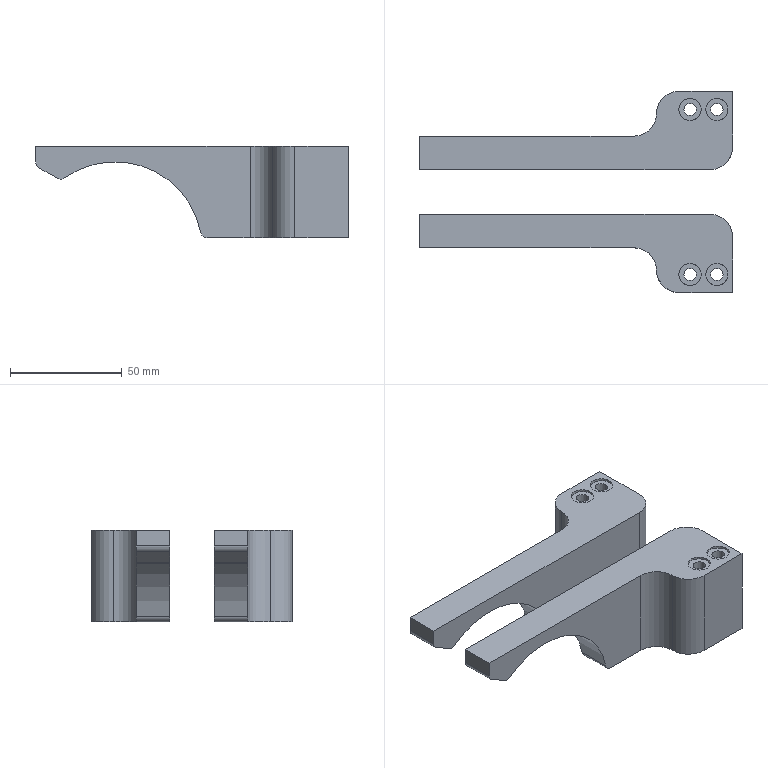NC program | NX | posted with a generic post | part box 140 x 90 x 41 mm
Lines 5892 to 6729 of 29499:
(FIXED_CONTOUR_COPY , TOOL : R4)
N11740 T08 M6
N11742 G54
N11744 G17 G0 G90 X6.198 Y17.997 S9500 M3
N11746 G43 Z30. H8
N11748 Z4.4
N11750 G94 G1 Z0.371 F3000.
N11752 X6.29 Y17.904 Z0.209
N11754 X6.41 Y17.785 Z0.086
N11756 X6.548 Y17.647 Z0.011
N11758 X6.695 Y17.5 Z-0.011
N11760 X6.831 Y17.363 Z-0.006
N11762 Y17.227 Z-0.004
N11764 X6.558 Y17.5 Z-0.014
N11766 X6.421 Z-0.017
N11768 X6.831 Y17.09 Z-0.004
N11770 Y16.954
N11772 X6.589 Y17.196 Z-0.009
N11774 X6.427 Y17.358 Z-0.015
N11776 X6.285 Y17.5 Z-0.028
N11778 X6.148 Z-0.039
N11780 X6.427 Y17.221 Z-0.013
N11782 X6.831 Y16.817 Z-0.004
N11784 Y16.682
N11786 X6.427 Y17.086 Z-0.013
N11788 X6.145 Y17.368 Z-0.037
N11790 X6.013 Y17.5 Z-0.055
N11792 X5.877 Z-0.071
N11794 X6.181 Y17.196 Z-0.032
N11796 X6.427 Y16.95 Z-0.013
N11798 X6.831 Y16.546 Z-0.004
N11800 Y16.409
N11802 X6.427 Y16.813 Z-0.013
N11804 X6.145 Y17.095 Z-0.035
N11806 X5.863 Y17.377 Z-0.07
N11808 X5.74 Y17.5 Z-0.092
N11810 X5.605 Z-0.115
N11812 X5.863 Y17.241 Z-0.068
N11814 X6.145 Y16.959 Z-0.035
N11816 X6.427 Y16.678 Z-0.013
N11818 X6.831 Y16.274 Z-0.004
N11820 Y16.14
N11822 X6.427 Y16.544 Z-0.013
N11824 X6.145 Y16.826 Z-0.035
N11826 X5.863 Y17.108 Z-0.068
N11828 X5.582 Y17.389 Z-0.117
N11830 X5.471 Y17.5 Z-0.144
N11832 X5.336 Z-0.174
N11834 X5.582 Y17.254 Z-0.115
N11836 X5.863 Y16.973 Z-0.068
N11838 X6.145 Y16.691 Z-0.035
N11840 X6.427 Y16.409 Z-0.013
N11842 X6.831 Y16.005 Z-0.004
N11844 Y15.87
N11846 X6.427 Y16.274 Z-0.013
N11848 X6.145 Y16.555 Z-0.035
N11850 X5.863 Y16.837 Z-0.068
N11852 X5.582 Y17.119 Z-0.114
N11854 X5.201 Y17.5 Z-0.206
N11856 X5.065 Z-0.238
N11858 X5.369 Y17.196 Z-0.163
N11860 X5.582 Y16.983 Z-0.114
N11862 X5.863 Y16.702 Z-0.068
N11864 X6.145 Y16.42 Z-0.035
N11866 X6.427 Y16.138 Z-0.013
N11868 X6.831 Y15.734 Z-0.004
N11870 Y15.599
N11872 X6.427 Y16.003 Z-0.013
N11874 X6.145 Y16.285 Z-0.035
N11876 X5.863 Y16.567 Z-0.068
N11878 X5.582 Y16.848 Z-0.114
N11880 X5.234 Y17.196 Z-0.194
N11882 X5.018 Y17.412 Z-0.247
N11884 X4.93 Y17.5 Z-0.273
N11886 X4.795 Z-0.309
N11888 X5.018 Y17.277 Z-0.245
N11890 X5.3 Y16.996 Z-0.178
N11892 X5.582 Y16.714 Z-0.114
N11894 X5.863 Y16.432 Z-0.068
N11896 X6.145 Y16.15 Z-0.035
N11898 X6.427 Y15.869 Z-0.013
N11900 X6.831 Y15.464 Z-0.004
N11902 Y15.333
N11904 X6.427 Y15.737 Z-0.013
N11906 X6.145 Y16.018 Z-0.035
N11908 X5.863 Y16.3 Z-0.068
N11910 X5.582 Y16.582 Z-0.114
N11912 X5.018 Y17.145 Z-0.244
N11914 X4.736 Y17.427 Z-0.324
N11916 X4.664 Y17.5 Z-0.351
N11918 X4.531 Z-0.398
N11920 X4.736 Y17.295 Z-0.322
N11922 X5.018 Y17.013 Z-0.244
N11924 X5.582 Y16.449 Z-0.114
N11926 X5.863 Y16.168 Z-0.068
N11928 X6.145 Y15.886 Z-0.035
N11930 X6.427 Y15.604 Z-0.013
N11932 X6.831 Y15.2 Z-0.004
N11934 Y15.067
N11936 X6.427 Y15.471 Z-0.013
N11938 X6.145 Y15.753 Z-0.035
N11940 X5.863 Y16.034 Z-0.068
N11942 X5.582 Y16.316 Z-0.114
N11944 X5.018 Y16.88 Z-0.244
N11946 X4.736 Y17.161 Z-0.321
N11948 X4.455 Y17.443 Z-0.424
N11950 X4.398 Y17.5 Z-0.448
N11952 X4.265 Z-0.501
N11954 X4.455 Y17.311 Z-0.422
N11956 X4.736 Y17.029 Z-0.321
N11958 X5.018 Y16.747 Z-0.244
N11960 X5.582 Y16.184 Z-0.114
N11962 X5.863 Y15.902 Z-0.068
N11964 X6.145 Y15.62 Z-0.035
N11966 X6.427 Y15.338 Z-0.013
N11968 X6.831 Y14.934 Z-0.004
N11970 Y14.802
N11972 X6.427 Y15.206 Z-0.013
N11974 X6.145 Y15.488 Z-0.035
N11976 X5.863 Y15.77 Z-0.068
N11978 X5.582 Y16.051 Z-0.114
N11980 X5.018 Y16.615 Z-0.244
N11982 X4.736 Y16.897 Z-0.321
N11984 X4.437 Y17.196 Z-0.427
N11986 X4.133 Y17.5 Z-0.555
N11988 X4.002 Z-0.608
N11990 X4.306 Y17.196 Z-0.48
N11992 X4.455 Y17.047 Z-0.42
N11994 X4.736 Y16.766 Z-0.321
N11996 X5.018 Y16.484 Z-0.244
N11998 X5.582 Y15.92 Z-0.114
N12000 X5.863 Y15.639 Z-0.068
N12002 X6.145 Y15.357 Z-0.035
N12004 X6.427 Y15.075 Z-0.013
N12006 X6.831 Y14.671 Z-0.004
N12008 Y14.541
N12010 X6.427 Y14.945 Z-0.013
N12012 X6.145 Y15.227 Z-0.035
N12014 X5.863 Y15.509 Z-0.068
N12016 X5.582 Y15.791 Z-0.114
N12018 X5.018 Y16.354 Z-0.244
N12020 X4.736 Y16.636 Z-0.321
N12022 X4.455 Y16.918 Z-0.42
N12024 X4.176 Y17.196 Z-0.532
N12026 X3.891 Y17.481 Z-0.654
N12028 X3.872 Y17.5 Z-0.663
N12030 X3.744 Z-0.726
N12032 X3.891 Y17.353 Z-0.652
N12034 X4.173 Y17.071 Z-0.534
N12036 X4.455 Y16.79 Z-0.42
N12038 X4.736 Y16.508 Z-0.321
N12040 X5.018 Y16.226 Z-0.244
N12042 X5.582 Y15.663 Z-0.114
N12044 X5.863 Y15.381 Z-0.068
N12046 X6.145 Y15.099 Z-0.035
N12048 X6.427 Y14.817 Z-0.013
N12050 X6.831 Y14.413 Z-0.004
N12052 Y14.283
N12054 X6.427 Y14.687 Z-0.013
N12056 X6.145 Y14.969 Z-0.035
N12058 X5.863 Y15.251 Z-0.068
N12060 X5.582 Y15.532 Z-0.114
N12062 X5.02 Y16.094 Z-0.244
N12064 X4.736 Y16.378 Z-0.321
N12066 X4.455 Y16.659 Z-0.42
N12068 X3.891 Y17.223 Z-0.65
N12070 X3.614 Y17.5 Z-0.785
N12072 X3.487 Z-0.858
N12074 X3.609 Y17.377 Z-0.787
N12076 X3.891 Y17.096 Z-0.649
N12078 X4.455 Y16.532 Z-0.42
N12080 X4.736 Y16.25 Z-0.321
N12082 X5.018 Y15.969 Z-0.244
N12084 X5.582 Y15.405 Z-0.114
N12086 X5.863 Y15.123 Z-0.068
N12088 X6.145 Y14.842 Z-0.035
N12090 X6.427 Y14.56 Z-0.013
N12092 X6.831 Y14.156 Z-0.004
N12094 Y14.032
N12096 X6.427 Y14.437 Z-0.013
N12098 X6.145 Y14.718 Z-0.035
N12100 X5.863 Y15. Z-0.068
N12102 X5.582 Y15.282 Z-0.114
N12104 X5.018 Y15.845 Z-0.244
N12106 X4.736 Y16.127 Z-0.321
N12108 X4.455 Y16.409 Z-0.42
N12110 X3.891 Y16.972 Z-0.649
N12112 X3.609 Y17.254 Z-0.787
N12114 X3.363 Y17.5 Z-0.93
N12116 X3.237 Z-1.004
N12118 X3.327 Y17.41 Z-0.95
N12120 X3.609 Y17.128 Z-0.787
N12122 X3.891 Y16.846 Z-0.649
N12124 X4.455 Y16.283 Z-0.42
N12126 X4.736 Y16.001 Z-0.321
N12128 X5.018 Y15.719 Z-0.244
N12130 X5.582 Y15.156 Z-0.114
N12132 X5.863 Y14.874 Z-0.068
N12134 X6.145 Y14.592 Z-0.035
N12136 X6.427 Y14.31 Z-0.013
N12138 X6.831 Y13.906 Z-0.004
N12140 Y13.779
N12142 X6.427 Y14.183 Z-0.013
N12144 X6.145 Y14.465 Z-0.035
N12146 X5.863 Y14.747 Z-0.068
N12148 X5.582 Y15.029 Z-0.114
N12150 X5.018 Y15.592 Z-0.244
N12152 X4.736 Y15.874 Z-0.321
N12154 X4.455 Y16.156 Z-0.42
N12156 X3.891 Y16.719 Z-0.649
N12158 X3.609 Y17.001 Z-0.787
N12160 X3.327 Y17.283 Z-0.95
N12162 X3.11 Y17.5 Z-1.08
N12164 X3.046 Z-1.118
N12166 X2.985 Z-1.16
N12168 X3.046 Y17.439 Z-1.117
N12170 X3.327 Y17.157 Z-0.95
N12172 X3.609 Y16.875 Z-0.787
N12174 X3.891 Y16.593 Z-0.649
N12176 X4.455 Y16.03 Z-0.42
N12178 X4.736 Y15.748 Z-0.321
N12180 X5.018 Y15.466 Z-0.244
N12182 X5.582 Y14.903 Z-0.114
N12184 X5.863 Y14.621 Z-0.068
N12186 X6.145 Y14.339 Z-0.035
N12188 X6.427 Y14.058 Z-0.013
N12190 X6.831 Y13.653 Z-0.004
N12192 Y13.531
N12194 X6.427 Y13.935 Z-0.013
N12196 X6.145 Y14.217 Z-0.035
N12198 X5.863 Y14.499 Z-0.068
N12200 X5.582 Y14.781 Z-0.114
N12202 X5.018 Y15.344 Z-0.244
N12204 X4.736 Y15.626 Z-0.321
N12206 X4.455 Y15.908 Z-0.42
N12208 X3.891 Y16.471 Z-0.649
N12210 X3.609 Y16.753 Z-0.787
N12212 X3.327 Y17.035 Z-0.95
N12214 X3.046 Y17.317 Z-1.117
N12216 X2.967 Y17.395 Z-1.169
N12218 X2.862 Y17.5 Z-1.243
N12220 X2.764 Z-1.308
N12222 X2.74 Z-1.327
N12224 X2.764 Y17.476 Z-1.308
N12226 X2.858 Y17.381 Z-1.244
N12228 X2.905 Y17.335 Z-1.21
N12230 X3.046 Y17.194 Z-1.117
N12232 X3.327 Y16.912 Z-0.95
N12234 X3.609 Y16.631 Z-0.787
N12236 X3.891 Y16.349 Z-0.649
N12238 X4.455 Y15.785 Z-0.42
N12240 X4.736 Y15.504 Z-0.321
N12242 X5.018 Y15.222 Z-0.244
N12244 X5.582 Y14.658 Z-0.114
N12246 X5.863 Y14.376 Z-0.068
N12248 X6.145 Y14.095 Z-0.035
N12250 X6.427 Y13.813 Z-0.013
N12252 X6.831 Y13.409 Z-0.004
N12254 Y13.289
N12256 X6.427 Y13.693 Z-0.013
N12258 X6.145 Y13.975 Z-0.035
N12260 X5.863 Y14.257 Z-0.068
N12262 X5.582 Y14.539 Z-0.114
N12264 X5.018 Y15.102 Z-0.244
N12266 X4.736 Y15.384 Z-0.321
N12268 X4.455 Y15.666 Z-0.42
N12270 X3.891 Y16.229 Z-0.649
N12272 X3.609 Y16.511 Z-0.787
N12274 X3.327 Y16.793 Z-0.95
N12276 X3.046 Y17.075 Z-1.117
N12278 X2.845 Y17.275 Z-1.25
N12280 X2.764 Y17.356 Z-1.306
N12282 X2.62 Y17.5 Z-1.422
N12284 X2.502 Z-1.512
N12286 X2.764 Y17.238 Z-1.304
N12288 X3.046 Y16.956 Z-1.117
N12290 X3.327 Y16.675 Z-0.95
N12292 X3.609 Y16.393 Z-0.787
N12294 X3.891 Y16.111 Z-0.649
N12296 X4.455 Y15.548 Z-0.42
N12298 X4.736 Y15.266 Z-0.321
N12300 X5.02 Y14.982 Z-0.244
N12302 X5.582 Y14.42 Z-0.114
N12304 X5.863 Y14.139 Z-0.068
N12306 X6.145 Y13.857 Z-0.035
N12308 X6.427 Y13.575 Z-0.013
N12310 X6.831 Y13.171 Z-0.004
N12312 Y13.057
N12314 X6.427 Y13.461 Z-0.013
N12316 X6.145 Y13.743 Z-0.035
N12318 X5.863 Y14.025 Z-0.068
N12320 X5.582 Y14.307 Z-0.114
N12322 X5.018 Y14.87 Z-0.244
N12324 X4.736 Y15.152 Z-0.321
N12326 X4.455 Y15.434 Z-0.42
N12328 X3.891 Y15.997 Z-0.649
N12330 X3.609 Y16.279 Z-0.787
N12332 X3.327 Y16.561 Z-0.95
N12334 X3.046 Y16.843 Z-1.117
N12336 X2.764 Y17.124 Z-1.303
N12338 X2.451 Y17.438 Z-1.551
N12340 X2.388 Y17.5 Z-1.604
N12342 X2.27 Z-1.701
N12344 X2.482 Y17.288 Z-1.525
N12346 X2.764 Y17.006 Z-1.303
N12348 X3.046 Y16.724 Z-1.117
N12350 X3.327 Y16.442 Z-0.95
N12352 X3.609 Y16.161 Z-0.787
N12354 X3.891 Y15.879 Z-0.649
N12356 X4.455 Y15.315 Z-0.42
N12358 X4.736 Y15.033 Z-0.321
N12360 X5.018 Y14.752 Z-0.244
N12362 X5.582 Y14.188 Z-0.114
N12364 X5.863 Y13.906 Z-0.068
N12366 X6.145 Y13.625 Z-0.035
N12368 X6.427 Y13.343 Z-0.013
N12370 X6.831 Y12.939 Z-0.004
N12372 Y12.82
N12374 X6.427 Y13.224 Z-0.013
N12376 X6.145 Y13.505 Z-0.035
N12378 X5.863 Y13.787 Z-0.068
N12380 X5.582 Y14.069 Z-0.114
N12382 X5.018 Y14.633 Z-0.244
N12384 X4.736 Y14.914 Z-0.321
N12386 X4.455 Y15.196 Z-0.42
N12388 X3.891 Y15.76 Z-0.649
N12390 X3.609 Y16.041 Z-0.787
N12392 X3.327 Y16.323 Z-0.95
N12394 X3.046 Y16.605 Z-1.117
N12396 X2.764 Y16.887 Z-1.303
N12398 X2.482 Y17.168 Z-1.525
N12400 X2.189 Y17.461 Z-1.766
N12402 X2.151 Y17.5 Z-1.803
N12404 X2.032 Z-1.907
N12406 X2.06 Y17.472 Z-1.879
N12408 X2.2 Y17.331 Z-1.757
N12410 X2.482 Y17.049 Z-1.525
N12412 X2.764 Y16.768 Z-1.303
N12414 X3.046 Y16.486 Z-1.117
N12416 X3.327 Y16.204 Z-0.95
N12418 X3.609 Y15.922 Z-0.787
N12420 X3.891 Y15.641 Z-0.649
N12422 X4.455 Y15.077 Z-0.42
N12424 X4.736 Y14.795 Z-0.321
N12426 X5.018 Y14.514 Z-0.244
N12428 X5.582 Y13.95 Z-0.114
N12430 X5.863 Y13.668 Z-0.068
N12432 X6.145 Y13.386 Z-0.035
N12434 X6.427 Y13.105 Z-0.013
N12436 X6.831 Y12.701 Z-0.004
N12438 Y12.587
N12440 X6.427 Y12.991 Z-0.013
N12442 X6.145 Y13.272 Z-0.035
N12444 X5.863 Y13.554 Z-0.068
N12446 X5.582 Y13.836 Z-0.114
N12448 X5.018 Y14.4 Z-0.244
N12450 X4.736 Y14.681 Z-0.321
N12452 X4.455 Y14.963 Z-0.42
N12454 X3.891 Y15.527 Z-0.649
N12456 X3.609 Y15.808 Z-0.787
N12458 X3.329 Y16.089 Z-0.949
N12460 X3.046 Y16.372 Z-1.117
N12462 X2.764 Y16.654 Z-1.303
N12464 X2.482 Y16.935 Z-1.525
N12466 X2.178 Y17.239 Z-1.776
N12468 X1.979 Y17.439 Z-1.955
N12470 X1.917 Y17.5 Z-2.016
N12472 X1.811 Z-2.132
N12474 X1.919 Y17.392 Z-2.014
N12476 X1.985 Y17.326 Z-1.951
N12478 X2.2 Y17.11 Z-1.757
N12480 X2.482 Y16.828 Z-1.525
N12482 X2.764 Y16.547 Z-1.303
N12484 X3.046 Y16.265 Z-1.117
N12486 X3.327 Y15.983 Z-0.95
N12488 X3.609 Y15.701 Z-0.787
N12490 X3.891 Y15.419 Z-0.649
N12492 X4.455 Y14.856 Z-0.42
N12494 X4.736 Y14.574 Z-0.321
N12496 X5.018 Y14.292 Z-0.244
N12498 X5.582 Y13.729 Z-0.114
N12500 X5.863 Y13.447 Z-0.068
N12502 X6.145 Y13.165 Z-0.035
N12504 X6.427 Y12.884 Z-0.013
N12506 X6.831 Y12.479 Z-0.004
N12508 Y12.371
N12510 X6.427 Y12.775 Z-0.013
N12512 X6.145 Y13.057 Z-0.035
N12514 X5.863 Y13.339 Z-0.068
N12516 X5.582 Y13.621 Z-0.114
N12518 X5.018 Y14.184 Z-0.244
N12520 X4.736 Y14.466 Z-0.321
N12522 X4.455 Y14.748 Z-0.42
N12524 X3.891 Y15.311 Z-0.649
N12526 X3.609 Y15.593 Z-0.787
N12528 X3.327 Y15.875 Z-0.95
N12530 X3.046 Y16.156 Z-1.117
N12532 X2.764 Y16.438 Z-1.303
N12534 X2.482 Y16.72 Z-1.525
N12536 X2.2 Y17.002 Z-1.757
N12538 X1.919 Y17.284 Z-2.014
N12540 X1.702 Y17.5 Z-2.25
N12542 X1.593 Z-2.37
N12544 X1.637 Y17.456 Z-2.32
N12546 X1.919 Y17.175 Z-2.014
N12548 X2.2 Y16.893 Z-1.757
N12550 X2.482 Y16.611 Z-1.525
N12552 X2.764 Y16.329 Z-1.303
N12554 X3.046 Y16.048 Z-1.117
N12556 X3.327 Y15.766 Z-0.95
N12558 X3.609 Y15.484 Z-0.787
N12560 X3.891 Y15.202 Z-0.649
N12562 X4.455 Y14.639 Z-0.42
N12564 X4.736 Y14.357 Z-0.321
N12566 X5.018 Y14.075 Z-0.244
N12568 X5.582 Y13.512 Z-0.114
N12570 X5.863 Y13.23 Z-0.068
N12572 X6.145 Y12.948 Z-0.035
N12574 X6.427 Y12.666 Z-0.013
N12576 X6.831 Y12.262 Z-0.004
N12578 Y12.154
N12580 X6.427 Y12.558 Z-0.013
N12582 X6.145 Y12.84 Z-0.035
N12584 X5.863 Y13.121 Z-0.068
N12586 X5.582 Y13.403 Z-0.114
N12588 X5.018 Y13.967 Z-0.244
N12590 X4.736 Y14.249 Z-0.321
N12592 X4.455 Y14.53 Z-0.42
N12594 X3.891 Y15.094 Z-0.649
N12596 X3.609 Y15.376 Z-0.787
N12598 X3.327 Y15.657 Z-0.95
N12600 X3.046 Y15.939 Z-1.117
N12602 X2.764 Y16.221 Z-1.303
N12604 X2.482 Y16.503 Z-1.525
N12606 X2.2 Y16.785 Z-1.757
N12608 X1.919 Y17.066 Z-2.014
N12610 X1.637 Y17.348 Z-2.32
N12612 X1.485 Y17.5 Z-2.492
N12614 X1.378 Z-2.614
N12616 X1.418 Y17.46 Z-2.566
N12618 X1.637 Y17.241 Z-2.32
N12620 X1.919 Y16.96 Z-2.014
N12622 X2.2 Y16.678 Z-1.757
N12624 X2.482 Y16.396 Z-1.525
N12626 X2.764 Y16.114 Z-1.303
N12628 X3.046 Y15.833 Z-1.117
N12630 X3.333 Y15.546 Z-0.946
N12632 X3.609 Y15.269 Z-0.787
N12634 X3.891 Y14.987 Z-0.649
N12636 X4.455 Y14.424 Z-0.42
N12638 X4.736 Y14.142 Z-0.321
N12640 X5.018 Y13.86 Z-0.244
N12642 X5.582 Y13.297 Z-0.114
N12644 X5.863 Y13.015 Z-0.068
N12646 X6.145 Y12.733 Z-0.035
N12648 X6.427 Y12.451 Z-0.013
N12650 X6.831 Y12.047 Z-0.004
N12652 Y11.952
N12654 X6.427 Y12.356 Z-0.013
N12656 X6.145 Y12.638 Z-0.035
N12658 X5.863 Y12.919 Z-0.068
N12660 X5.582 Y13.201 Z-0.114
N12662 X5.018 Y13.765 Z-0.244
N12664 X4.736 Y14.046 Z-0.321
N12666 X4.455 Y14.328 Z-0.42
N12668 X3.891 Y14.892 Z-0.649
N12670 X3.609 Y15.174 Z-0.787
N12672 X3.327 Y15.455 Z-0.95
N12674 X3.046 Y15.737 Z-1.117
N12676 X2.764 Y16.019 Z-1.303
N12678 X2.482 Y16.301 Z-1.525
N12680 X2.2 Y16.582 Z-1.757
N12682 X1.919 Y16.864 Z-2.014
N12684 X1.637 Y17.146 Z-2.32
N12686 X1.4 Y17.383 Z-2.588
N12688 X1.333 Y17.449 Z-2.669
N12690 X1.283 Y17.5 Z-2.742
N12692 X1.214 Z-2.83
N12694 X1.181 Z-2.879
N12696 X1.214 Y17.467 Z-2.83
N12698 X1.269 Y17.412 Z-2.757
N12700 X1.301 Y17.38 Z-2.711
N12702 X1.355 Y17.326 Z-2.641
N12704 X1.637 Y17.044 Z-2.32
N12706 X1.919 Y16.763 Z-2.014
N12708 X2.2 Y16.481 Z-1.757
N12710 X2.482 Y16.199 Z-1.525
N12712 X2.764 Y15.917 Z-1.303
N12714 X3.046 Y15.636 Z-1.117
N12716 X3.327 Y15.354 Z-0.95
N12718 X3.609 Y15.072 Z-0.787
N12720 X3.891 Y14.79 Z-0.649
N12722 X4.455 Y14.227 Z-0.42
N12724 X4.736 Y13.945 Z-0.321
N12726 X5.018 Y13.663 Z-0.244
N12728 X5.582 Y13.1 Z-0.114
N12730 X5.863 Y12.818 Z-0.068
N12732 X6.145 Y12.536 Z-0.035
N12734 X6.427 Y12.254 Z-0.013
N12736 X6.831 Y11.85 Z-0.004
N12738 Y11.749
N12740 X6.427 Y12.153 Z-0.013
N12742 X6.145 Y12.435 Z-0.035
N12744 X5.863 Y12.717 Z-0.068
N12746 X5.582 Y12.999 Z-0.114
N12748 X5.018 Y13.562 Z-0.244
N12750 X4.736 Y13.844 Z-0.321
N12752 X4.455 Y14.126 Z-0.42
N12754 X3.891 Y14.689 Z-0.649
N12756 X3.609 Y14.971 Z-0.787
N12758 X3.327 Y15.253 Z-0.95
N12760 X3.046 Y15.534 Z-1.117
N12762 X2.764 Y15.816 Z-1.303
N12764 X2.482 Y16.098 Z-1.525
N12766 X2.2 Y16.38 Z-1.757
N12768 X1.919 Y16.662 Z-2.014
N12770 X1.637 Y16.943 Z-2.32
N12772 X1.355 Y17.225 Z-2.641
N12774 X1.269 Y17.312 Z-2.753
N12776 X1.214 Y17.366 Z-2.827
N12778 X1.08 Y17.5 Z-3.027
N12780 X0.982 Z-3.177
N12782 X1.116 Y17.365 Z-2.97
N12784 X1.214 Y17.268 Z-2.825
N12786 X1.355 Y17.127 Z-2.641
N12788 X1.637 Y16.845 Z-2.32
N12790 X1.919 Y16.563 Z-2.014
N12792 X2.2 Y16.281 Z-1.757
N12794 X2.482 Y16. Z-1.525
N12796 X2.764 Y15.718 Z-1.303
N12798 X3.046 Y15.436 Z-1.117
N12800 X3.327 Y15.154 Z-0.95
N12802 X3.609 Y14.873 Z-0.787
N12804 X3.891 Y14.591 Z-0.649
N12806 X4.455 Y14.027 Z-0.42
N12808 X4.736 Y13.745 Z-0.321
N12810 X5.018 Y13.464 Z-0.244
N12812 X5.582 Y12.9 Z-0.114
N12814 X5.863 Y12.618 Z-0.068
N12816 X6.145 Y12.337 Z-0.035
N12818 X6.427 Y12.055 Z-0.013
N12820 X6.831 Y11.651 Z-0.004
N12822 Y11.555
N12824 X6.427 Y11.959 Z-0.013
N12826 X6.145 Y12.241 Z-0.035
N12828 X5.863 Y12.523 Z-0.068
N12830 X5.582 Y12.805 Z-0.114
N12832 X5.018 Y13.368 Z-0.244
N12834 X4.736 Y13.65 Z-0.321
N12836 X4.455 Y13.932 Z-0.42
N12838 X3.891 Y14.495 Z-0.649
N12840 X3.609 Y14.777 Z-0.787
N12842 X3.327 Y15.059 Z-0.95
N12844 X3.046 Y15.34 Z-1.117
N12846 X2.764 Y15.622 Z-1.303
N12848 X2.482 Y15.904 Z-1.525
N12850 X2.2 Y16.186 Z-1.757
N12852 X1.919 Y16.468 Z-2.014
N12854 X1.637 Y16.749 Z-2.32
N12856 X1.355 Y17.031 Z-2.641
N12858 X1.214 Y17.172 Z-2.823
N12860 X1.073 Y17.313 Z-3.032
N12862 X0.886 Y17.5 Z-3.323
N12864 X0.793 Z-3.465
N12866 X1.098 Y17.196 Z-2.994
N12868 X1.214 Y17.079 Z-2.823
N12870 X1.355 Y16.939 Z-2.641
N12872 X1.637 Y16.657 Z-2.32
N12874 X1.919 Y16.375 Z-2.014
N12876 X2.2 Y16.093 Z-1.757
N12878 X2.482 Y15.812 Z-1.525
N12880 X2.764 Y15.53 Z-1.303
N12882 X3.046 Y15.248 Z-1.117
N12884 X3.327 Y14.966 Z-0.95
N12886 X3.609 Y14.684 Z-0.787
N12888 X3.891 Y14.403 Z-0.649
N12890 X4.455 Y13.839 Z-0.42
N12892 X4.736 Y13.557 Z-0.321
N12894 X5.018 Y13.276 Z-0.244
N12896 X5.582 Y12.712 Z-0.114
N12898 X5.863 Y12.43 Z-0.068
N12900 X6.145 Y12.148 Z-0.035
N12902 X6.427 Y11.867 Z-0.013
N12904 X6.831 Y11.463 Z-0.004
N12906 Y11.377
N12908 X6.427 Y11.781 Z-0.013
N12910 X6.145 Y12.063 Z-0.035
N12912 X5.863 Y12.344 Z-0.068
N12914 X5.582 Y12.626 Z-0.114
N12916 X5.018 Y13.19 Z-0.244
N12918 X4.736 Y13.472 Z-0.321
N12920 X4.455 Y13.753 Z-0.42
N12922 X3.891 Y14.317 Z-0.649
N12924 X3.609 Y14.599 Z-0.787
N12926 X3.327 Y14.88 Z-0.95
N12928 X3.046 Y15.162 Z-1.117
N12930 X2.764 Y15.444 Z-1.303
N12932 X2.482 Y15.726 Z-1.525
N12934 X2.2 Y16.008 Z-1.757
N12936 X1.919 Y16.289 Z-2.014
N12938 X1.637 Y16.571 Z-2.32
N12940 X1.355 Y16.853 Z-2.641
N12942 X1.214 Y16.994 Z-2.823
N12944 X1.073 Y17.135 Z-3.029
N12946 X0.792 Y17.416 Z-3.466
N12948 X0.708 Y17.5 Z-3.615
N12950 X0.651 Z-3.715
N12952 X0.627 Z-3.765
N12954 X0.654 Y17.473 Z-3.707
N12956 X0.792 Y17.336 Z-3.466
N12958 X1.073 Y17.054 Z-3.029
N12960 X1.214 Y16.913 Z-2.823
N12962 X1.355 Y16.772 Z-2.641
N12964 X1.637 Y16.49 Z-2.32
N12966 X1.919 Y16.208 Z-2.014
N12968 X2.2 Y15.927 Z-1.757
N12970 X2.482 Y15.645 Z-1.525
N12972 X2.764 Y15.363 Z-1.303
N12974 X3.046 Y15.081 Z-1.117
N12976 X3.327 Y14.8 Z-0.95
N12978 X3.609 Y14.518 Z-0.787
N12980 X3.891 Y14.236 Z-0.649
N12982 X4.455 Y13.673 Z-0.42
N12984 X4.736 Y13.391 Z-0.321
N12986 X5.018 Y13.109 Z-0.244
N12988 X5.582 Y12.545 Z-0.114
N12990 X5.863 Y12.264 Z-0.068
N12992 X6.145 Y11.982 Z-0.035
N12994 X6.427 Y11.7 Z-0.013
N12996 X6.831 Y11.296 Z-0.004
N12998 Y11.219
N13000 X6.427 Y11.623 Z-0.013
N13002 X6.145 Y11.905 Z-0.035
N13004 X5.863 Y12.187 Z-0.068
N13006 X5.582 Y12.468 Z-0.114
N13008 X5.018 Y13.032 Z-0.244
N13010 X4.736 Y13.314 Z-0.321
N13012 X4.455 Y13.595 Z-0.42
N13014 X3.891 Y14.159 Z-0.649
N13016 X3.609 Y14.441 Z-0.787
N13018 X3.327 Y14.722 Z-0.95
N13020 X3.046 Y15.004 Z-1.117
N13022 X2.764 Y15.286 Z-1.303
N13024 X2.482 Y15.568 Z-1.525
N13026 X2.2 Y15.85 Z-1.757
N13028 X1.919 Y16.131 Z-2.014
N13030 X1.637 Y16.413 Z-2.32
N13032 X1.355 Y16.695 Z-2.641
N13034 X1.214 Y16.836 Z-2.823
N13036 X1.073 Y16.977 Z-3.029
N13038 X0.792 Y17.258 Z-3.466
N13040 X0.651 Y17.399 Z-3.714
N13042 X0.55 Y17.5 Z-3.928
N13044 X0.473 Z-4.095
N13046 X0.51 Y17.463 Z-4.01
N13048 X0.651 Y17.322 Z-3.714
N13050 X0.792 Y17.181 Z-3.466
N13052 X1.073 Y16.9 Z-3.029
N13054 X1.214 Y16.759 Z-2.823
N13056 X1.355 Y16.618 Z-2.641
N13058 X1.637 Y16.336 Z-2.32
N13060 X1.919 Y16.054 Z-2.014
N13062 X2.2 Y15.772 Z-1.757
N13064 X2.482 Y15.491 Z-1.525
N13066 X2.764 Y15.209 Z-1.303
N13068 X3.046 Y14.927 Z-1.117
N13070 X3.327 Y14.645 Z-0.95
N13072 X3.609 Y14.364 Z-0.787
N13074 X3.891 Y14.082 Z-0.649
N13076 X4.455 Y13.518 Z-0.42
N13078 X4.736 Y13.237 Z-0.321
N13080 X5.018 Y12.955 Z-0.244
N13082 X5.582 Y12.391 Z-0.114
N13084 X5.863 Y12.109 Z-0.068
N13086 X6.145 Y11.828 Z-0.035
N13088 X6.427 Y11.546 Z-0.013
N13090 X6.831 Y11.142 Z-0.004
N13092 Y11.066
N13094 X6.427 Y11.47 Z-0.013
N13096 X6.145 Y11.752 Z-0.035
N13098 X5.863 Y12.034 Z-0.068
N13100 X5.582 Y12.316 Z-0.114
N13102 X5.018 Y12.879 Z-0.244
N13104 X4.736 Y13.161 Z-0.321
N13106 X4.455 Y13.443 Z-0.42
N13108 X3.891 Y14.006 Z-0.649
N13110 X3.609 Y14.288 Z-0.787
N13112 X3.327 Y14.57 Z-0.95
N13114 X3.046 Y14.852 Z-1.117
N13116 X2.764 Y15.134 Z-1.303
N13118 X2.482 Y15.415 Z-1.525
N13120 X2.2 Y15.697 Z-1.757
N13122 X1.919 Y15.979 Z-2.014
N13124 X1.637 Y16.261 Z-2.32
N13126 X1.355 Y16.542 Z-2.641
N13128 X1.214 Y16.683 Z-2.823
N13130 X1.073 Y16.824 Z-3.029
N13132 X0.792 Y17.106 Z-3.466
N13134 X0.651 Y17.247 Z-3.714
N13136 X0.51 Y17.388 Z-4.01
N13138 X0.397 Y17.5 Z-4.263
N13140 X0.369 Z-4.326
N13142 X0.328 Z-4.429
N13144 X0.369 Y17.459 Z-4.324
N13146 X0.51 Y17.318 Z-4.01
N13148 X0.651 Y17.177 Z-3.714
N13150 X0.792 Y17.036 Z-3.466
N13152 X1.073 Y16.755 Z-3.029
N13154 X1.214 Y16.614 Z-2.823
N13156 X1.355 Y16.473 Z-2.641
N13158 X1.637 Y16.191 Z-2.32
N13160 X1.919 Y15.909 Z-2.014
N13162 X2.2 Y15.628 Z-1.757
N13164 X2.482 Y15.346 Z-1.525
N13166 X2.764 Y15.064 Z-1.303
N13168 X3.046 Y14.782 Z-1.117
N13170 X3.327 Y14.5 Z-0.95
N13172 X3.609 Y14.219 Z-0.787
N13174 X3.891 Y13.937 Z-0.649
N13176 X4.455 Y13.373 Z-0.42
N13178 X4.736 Y13.092 Z-0.321
N13180 X5.018 Y12.81 Z-0.244
N13182 X5.582 Y12.246 Z-0.114
N13184 X5.863 Y11.965 Z-0.068
N13186 X6.145 Y11.683 Z-0.035
N13188 X6.427 Y11.401 Z-0.013
N13190 X6.831 Y10.997 Z-0.004
N13192 Y10.929
N13194 X6.427 Y11.333 Z-0.013
N13196 X6.145 Y11.615 Z-0.035
N13198 X5.863 Y11.896 Z-0.068
N13200 X5.582 Y12.178 Z-0.114
N13202 X5.018 Y12.742 Z-0.244
N13204 X4.736 Y13.024 Z-0.321
N13206 X4.455 Y13.305 Z-0.42
N13208 X3.891 Y13.869 Z-0.649
N13210 X3.609 Y14.151 Z-0.787
N13212 X3.332 Y14.428 Z-0.947
N13214 X3.046 Y14.714 Z-1.117
N13216 X2.764 Y14.996 Z-1.303
N13218 X2.482 Y15.278 Z-1.525
N13220 X2.2 Y15.559 Z-1.757
N13222 X1.919 Y15.841 Z-2.014
N13224 X1.637 Y16.123 Z-2.32
N13226 X1.355 Y16.405 Z-2.641
N13228 X1.214 Y16.546 Z-2.823
N13230 X1.073 Y16.687 Z-3.029
N13232 X0.792 Y16.968 Z-3.466
N13234 X0.651 Y17.109 Z-3.714
N13236 X0.51 Y17.25 Z-4.01
N13238 X0.369 Y17.391 Z-4.324
N13240 X0.26 Y17.5 Z-4.599
N13242 X0.228 Z-4.679
N13244 X0.201 Z-4.772
N13246 X0.228 Y17.473 Z-4.676
N13248 X0.369 Y17.332 Z-4.324
N13250 X0.51 Y17.191 Z-4.01
N13252 X0.651 Y17.05 Z-3.714
N13254 X0.792 Y16.909 Z-3.466
N13256 X1.073 Y16.627 Z-3.029
N13258 X1.214 Y16.486 Z-2.823
N13260 X1.355 Y16.346 Z-2.641
N13262 X1.637 Y16.064 Z-2.32
N13264 X1.919 Y15.782 Z-2.014
N13266 X2.2 Y15.5 Z-1.757
N13268 X2.482 Y15.218 Z-1.525
N13270 X2.764 Y14.937 Z-1.303
N13272 X3.046 Y14.655 Z-1.117
N13274 X3.327 Y14.373 Z-0.95
N13276 X3.609 Y14.091 Z-0.787
N13278 X3.891 Y13.81 Z-0.649
N13280 X4.455 Y13.246 Z-0.42
N13282 X4.736 Y12.964 Z-0.321
N13284 X5.018 Y12.683 Z-0.244
N13286 X5.582 Y12.119 Z-0.114
N13288 X5.863 Y11.837 Z-0.068
N13290 X6.145 Y11.555 Z-0.035
N13292 X6.427 Y11.274 Z-0.013
N13294 X6.831 Y10.87 Z-0.004
N13296 Y10.816
N13298 X6.427 Y11.22 Z-0.013
N13300 X6.145 Y11.501 Z-0.035
N13302 X5.863 Y11.783 Z-0.068
N13304 X5.582 Y12.065 Z-0.114
N13306 X5.018 Y12.629 Z-0.244
N13308 X4.736 Y12.91 Z-0.321
N13310 X4.455 Y13.192 Z-0.42
N13312 X3.891 Y13.756 Z-0.649
N13314 X3.609 Y14.037 Z-0.787
N13316 X3.327 Y14.319 Z-0.95
N13318 X3.046 Y14.601 Z-1.117
N13320 X2.764 Y14.883 Z-1.303
N13322 X2.482 Y15.164 Z-1.525
N13324 X2.2 Y15.446 Z-1.757
N13326 X1.919 Y15.728 Z-2.014
N13328 X1.637 Y16.01 Z-2.32
N13330 X1.355 Y16.292 Z-2.641
N13332 X1.214 Y16.432 Z-2.823
N13334 X1.073 Y16.573 Z-3.029
N13336 X0.792 Y16.855 Z-3.466
N13338 X0.651 Y16.996 Z-3.714
N13340 X0.51 Y17.137 Z-4.01
N13342 X0.369 Y17.278 Z-4.324
N13344 X0.228 Y17.419 Z-4.677
N13346 X0.147 Y17.5 Z-4.957
N13348 X0.091 Z-5.145
N13350 X0.228 Y17.363 Z-4.677
N13352 X0.369 Y17.223 Z-4.324
N13354 X0.51 Y17.082 Z-4.01
N13356 X0.651 Y16.941 Z-3.714
N13358 X0.792 Y16.8 Z-3.466
N13360 X1.073 Y16.518 Z-3.029
N13362 X1.214 Y16.377 Z-2.823
N13364 X1.355 Y16.236 Z-2.641
N13366 X1.637 Y15.955 Z-2.32
N13368 X1.919 Y15.673 Z-2.014
N13370 X2.2 Y15.391 Z-1.757
N13372 X2.482 Y15.109 Z-1.525
N13374 X2.764 Y14.827 Z-1.303
N13376 X3.046 Y14.546 Z-1.117
N13378 X3.327 Y14.264 Z-0.95
N13380 X3.609 Y13.982 Z-0.787
N13382 X3.891 Y13.7 Z-0.649
N13384 X4.455 Y13.137 Z-0.42
N13386 X4.736 Y12.855 Z-0.321
N13388 X5.018 Y12.573 Z-0.244
N13390 X5.582 Y12.01 Z-0.114
N13392 X5.863 Y11.728 Z-0.068
N13394 X6.145 Y11.446 Z-0.035
N13396 X6.427 Y11.164 Z-0.013
N13398 X6.831 Y10.76 Z-0.004
N13400 Y10.707
N13402 X6.427 Y11.111 Z-0.013
N13404 X6.145 Y11.393 Z-0.035
N13406 X5.863 Y11.675 Z-0.068
N13408 X5.582 Y11.957 Z-0.114